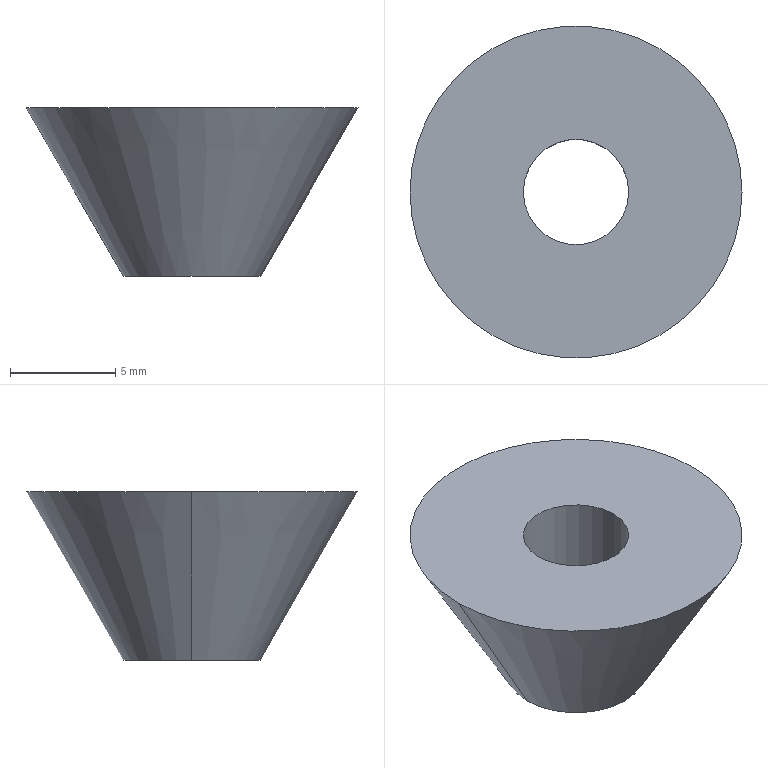Part | SolidWorks | features Extrusion 1, ICE 1 | 1 solid | 6 faces | box 15.738 x 15.738 x 8 mm | volume 664.377 mm3 | cylinder 2 | cone 2 | plane 2 | commonest cylinder face diameters 5 x2
STEP:
#1=CARTESIAN_POINT('',(2.5,0.,8.));
#2=VERTEX_POINT('',#1);
#3=CARTESIAN_POINT('',(-2.5,0.,8.));
#4=VERTEX_POINT('',#3);
#5=CARTESIAN_POINT('',(0.,0.,8.));
#6=DIRECTION('',(0.,0.,-1.));
#7=DIRECTION('',(-1.,0.,0.));
#8=AXIS2_PLACEMENT_3D('',#5,#6,#7);
#9=CIRCLE('',#8,2.5);
#10=EDGE_CURVE('',#2,#4,#9,.T.);
#11=ORIENTED_EDGE('',*,*,#10,.F.);
#12=CARTESIAN_POINT('',(2.5,0.,0.));
#13=VERTEX_POINT('',#12);
#14=CARTESIAN_POINT('',(2.5,0.,8.));
#15=DIRECTION('',(0.,0.,-1.));
#16=VECTOR('',#15,1000.);
#17=LINE('',#14,#16);
#18=EDGE_CURVE('',#2,#13,#17,.T.);
#19=ORIENTED_EDGE('',*,*,#18,.T.);
#20=CARTESIAN_POINT('',(-2.5,0.,0.));
#21=VERTEX_POINT('',#20);
#22=CARTESIAN_POINT('',(0.,0.,0.));
#23=DIRECTION('',(0.,0.,-1.));
#24=DIRECTION('',(-1.,0.,0.));
#25=AXIS2_PLACEMENT_3D('',#22,#23,#24);
#26=CIRCLE('',#25,2.5);
#27=EDGE_CURVE('',#13,#21,#26,.T.);
#28=ORIENTED_EDGE('',*,*,#27,.T.);
#29=CARTESIAN_POINT('',(-2.5,0.,8.));
#30=DIRECTION('',(0.,0.,-1.));
#31=VECTOR('',#30,1000.);
#32=LINE('',#29,#31);
#33=EDGE_CURVE('',#4,#21,#32,.T.);
#34=ORIENTED_EDGE('',*,*,#33,.F.);
#35=EDGE_LOOP('',(#11,#19,#28,#34));
#36=FACE_OUTER_BOUND('',#35,.T.);
#37=CARTESIAN_POINT('',(0.,0.,8.));
#38=DIRECTION('',(0.,0.,-1.));
#39=DIRECTION('',(-1.,0.,0.));
#40=AXIS2_PLACEMENT_3D('',#37,#38,#39);
#41=CYLINDRICAL_SURFACE('',#40,2.5);
#42=ADVANCED_FACE('',(#36),#41,.F.);
#43=CARTESIAN_POINT('',(3.25,0.,0.));
#44=VERTEX_POINT('',#43);
#45=CARTESIAN_POINT('',(-3.25,0.,0.));
#46=VERTEX_POINT('',#45);
#47=CARTESIAN_POINT('',(0.,0.,0.));
#48=DIRECTION('',(0.,0.,1.));
#49=DIRECTION('',(1.,0.,0.));
#50=AXIS2_PLACEMENT_3D('',#47,#48,#49);
#51=CIRCLE('',#50,3.25);
#52=EDGE_CURVE('',#44,#46,#51,.T.);
#53=ORIENTED_EDGE('',*,*,#52,.T.);
#54=CARTESIAN_POINT('',(-7.869,0.,8.));
#55=VERTEX_POINT('',#54);
#56=CARTESIAN_POINT('',(-3.25,0.,0.));
#57=DIRECTION('',(-0.5,0.,0.866));
#58=VECTOR('',#57,1000.);
#59=LINE('',#56,#58);
#60=EDGE_CURVE('',#46,#55,#59,.T.);
#61=ORIENTED_EDGE('',*,*,#60,.T.);
#62=CARTESIAN_POINT('',(7.869,0.,8.));
#63=VERTEX_POINT('',#62);
#64=CARTESIAN_POINT('',(0.,0.,8.));
#65=DIRECTION('',(0.,0.,1.));
#66=DIRECTION('',(1.,0.,0.));
#67=AXIS2_PLACEMENT_3D('',#64,#65,#66);
#68=CIRCLE('',#67,7.869);
#69=EDGE_CURVE('',#63,#55,#68,.T.);
#70=ORIENTED_EDGE('',*,*,#69,.F.);
#71=CARTESIAN_POINT('',(3.25,0.,0.));
#72=DIRECTION('',(0.5,0.,0.866));
#73=VECTOR('',#72,1000.);
#74=LINE('',#71,#73);
#75=EDGE_CURVE('',#44,#63,#74,.T.);
#76=ORIENTED_EDGE('',*,*,#75,.F.);
#77=EDGE_LOOP('',(#53,#61,#70,#76));
#78=FACE_OUTER_BOUND('',#77,.T.);
#79=CARTESIAN_POINT('',(0.,0.,0.));
#80=DIRECTION('',(0.,0.,1.));
#81=DIRECTION('',(1.,0.,0.));
#82=AXIS2_PLACEMENT_3D('',#79,#80,#81);
#83=CONICAL_SURFACE('',#82,3.25,0.5236);
#84=ADVANCED_FACE('',(#78),#83,.T.);
#85=ORIENTED_EDGE('',*,*,#60,.F.);
#86=CARTESIAN_POINT('',(0.,0.,0.));
#87=DIRECTION('',(0.,0.,1.));
#88=DIRECTION('',(1.,0.,0.));
#89=AXIS2_PLACEMENT_3D('',#86,#87,#88);
#90=CIRCLE('',#89,3.25);
#91=EDGE_CURVE('',#46,#44,#90,.T.);
#92=ORIENTED_EDGE('',*,*,#91,.T.);
#93=ORIENTED_EDGE('',*,*,#75,.T.);
#94=CARTESIAN_POINT('',(0.,0.,8.));
#95=DIRECTION('',(0.,0.,1.));
#96=DIRECTION('',(1.,0.,0.));
#97=AXIS2_PLACEMENT_3D('',#94,#95,#96);
#98=CIRCLE('',#97,7.869);
#99=EDGE_CURVE('',#55,#63,#98,.T.);
#100=ORIENTED_EDGE('',*,*,#99,.F.);
#101=EDGE_LOOP('',(#85,#92,#93,#100));
#102=FACE_OUTER_BOUND('',#101,.T.);
#103=CARTESIAN_POINT('',(0.,0.,0.));
#104=DIRECTION('',(0.,0.,1.));
#105=DIRECTION('',(1.,0.,0.));
#106=AXIS2_PLACEMENT_3D('',#103,#104,#105);
#107=CONICAL_SURFACE('',#106,3.25,0.5236);
#108=ADVANCED_FACE('',(#102),#107,.T.);
#109=CARTESIAN_POINT('',(0.,0.,8.));
#110=DIRECTION('',(0.,0.,-1.));
#111=DIRECTION('',(-1.,0.,0.));
#112=AXIS2_PLACEMENT_3D('',#109,#110,#111);
#113=CIRCLE('',#112,2.5);
#114=EDGE_CURVE('',#4,#2,#113,.T.);
#115=ORIENTED_EDGE('',*,*,#114,.T.);
#116=ORIENTED_EDGE('',*,*,#10,.T.);
#117=EDGE_LOOP('',(#115,#116));
#118=FACE_BOUND('',#117,.T.);
#119=ORIENTED_EDGE('',*,*,#69,.T.);
#120=ORIENTED_EDGE('',*,*,#99,.T.);
#121=EDGE_LOOP('',(#119,#120));
#122=FACE_OUTER_BOUND('',#121,.T.);
#123=CARTESIAN_POINT('',(0.,0.,8.));
#124=DIRECTION('',(0.,0.,1.));
#125=DIRECTION('',(1.,0.,0.));
#126=AXIS2_PLACEMENT_3D('',#123,#124,#125);
#127=PLANE('',#126);
#128=ADVANCED_FACE('',(#118,#122),#127,.T.);
#129=CARTESIAN_POINT('',(0.,0.,0.));
#130=DIRECTION('',(0.,0.,-1.));
#131=DIRECTION('',(-1.,0.,0.));
#132=AXIS2_PLACEMENT_3D('',#129,#130,#131);
#133=CIRCLE('',#132,2.5);
#134=EDGE_CURVE('',#21,#13,#133,.T.);
#135=ORIENTED_EDGE('',*,*,#134,.F.);
#136=ORIENTED_EDGE('',*,*,#27,.F.);
#137=EDGE_LOOP('',(#135,#136));
#138=FACE_BOUND('',#137,.T.);
#139=ORIENTED_EDGE('',*,*,#52,.F.);
#140=ORIENTED_EDGE('',*,*,#91,.F.);
#141=EDGE_LOOP('',(#139,#140));
#142=FACE_OUTER_BOUND('',#141,.T.);
#143=CARTESIAN_POINT('',(0.,0.,0.));
#144=DIRECTION('',(0.,0.,1.));
#145=DIRECTION('',(1.,0.,0.));
#146=AXIS2_PLACEMENT_3D('',#143,#144,#145);
#147=PLANE('',#146);
#148=ADVANCED_FACE('',(#138,#142),#147,.F.);
#149=ORIENTED_EDGE('',*,*,#18,.F.);
#150=ORIENTED_EDGE('',*,*,#114,.F.);
#151=ORIENTED_EDGE('',*,*,#33,.T.);
#152=ORIENTED_EDGE('',*,*,#134,.T.);
#153=EDGE_LOOP('',(#149,#150,#151,#152));
#154=FACE_OUTER_BOUND('',#153,.T.);
#155=CARTESIAN_POINT('',(0.,0.,8.));
#156=DIRECTION('',(0.,0.,-1.));
#157=DIRECTION('',(-1.,0.,0.));
#158=AXIS2_PLACEMENT_3D('',#155,#156,#157);
#159=CYLINDRICAL_SURFACE('',#158,2.5);
#160=ADVANCED_FACE('',(#154),#159,.F.);
#161=CLOSED_SHELL('',(#42,#84,#108,#128,#148,#160));
#162=MANIFOLD_SOLID_BREP('',#161);
#163=CARTESIAN_POINT('',(0.,0.,0.));
#164=DIRECTION('',(0.,0.,1.));
#165=DIRECTION('',(1.,0.,0.));
#166=AXIS2_PLACEMENT_3D('',#163,#164,#165);
#167=(LENGTH_UNIT()NAMED_UNIT(*)SI_UNIT(.MILLI.,.METRE.));
#168=UNCERTAINTY_MEASURE_WITH_UNIT(LENGTH_MEASURE(0.00001),#167,'','');
#169=(NAMED_UNIT(*)PLANE_ANGLE_UNIT()SI_UNIT($,.RADIAN.));
#170=(NAMED_UNIT(*)SI_UNIT($,.STERADIAN.)SOLID_ANGLE_UNIT());
#171=(GEOMETRIC_REPRESENTATION_CONTEXT(3)GLOBAL_UNCERTAINTY_ASSIGNED_CONTEXT((#168))GLOBAL_UNIT_ASSIGNED_CONTEXT((#167,#169,#170))REPRESENTATION_CONTEXT('',''));
#172=ADVANCED_BREP_SHAPE_REPRESENTATION('',(#162,#166),#171);